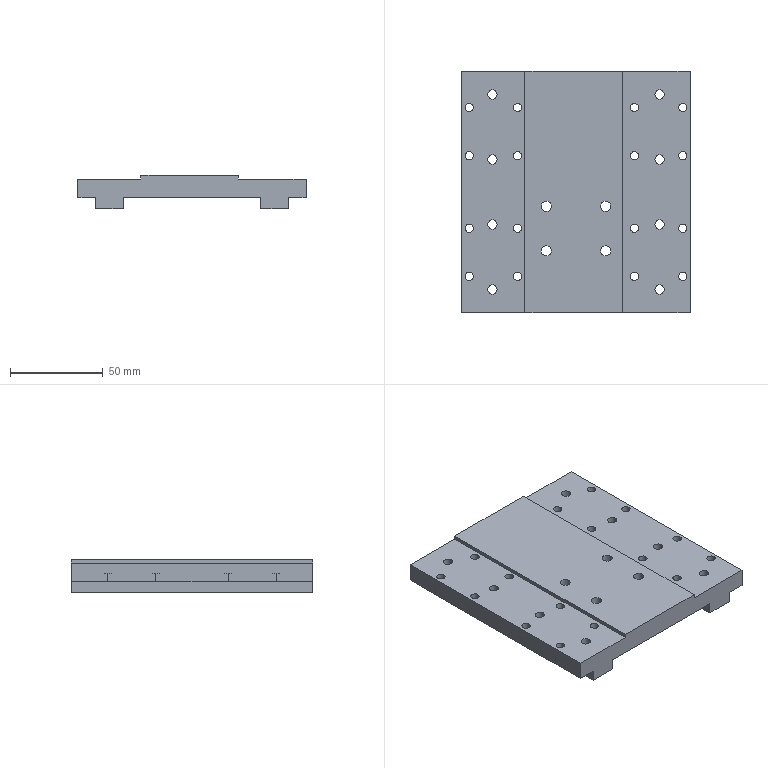NC program | NX | posted with a generic post | part box 123 x 130 x 18 mm
Whole program:
N10 G17 G21 G94 G90
(FLOOR_WALL_1_COPY , TOOL : D10)
N12 T15 M6
N14 G54
N16 G17 G0 G90 X4.33 Y-68. S9500 M3
N18 G43 Z30. H15
N20 Z0.517
N22 G94 G1 Z-0.983 F3000.
N24 X0.866 Y-62.
N26 G3 X0. Y-61.5 R1.
N28 G1 X-65.
N30 Y-57.1
N32 X65.
N34 Y-61.5
N36 X0.
N38 G3 X-0.866 Y-62. R1.
N40 G1 X-4.33 Y-68.
N42 Z0.517
N44 G0 X4.33 Z-0.467
N46 G1 Z-1.967
N48 X0.866 Y-62.
N50 G3 X0. Y-61.5 R1.
N52 G1 X-65.
N54 Y-57.1
N56 X65.
N58 Y-61.5
N60 X0.
N62 G3 X-0.866 Y-62. R1.
N64 G1 X-4.33 Y-68.
N66 Z-0.467
N68 G0 X4.33 Z-1.45
N70 G1 Z-2.95
N72 X0.866 Y-62.
N74 G3 X0. Y-61.5 R1.
N76 G1 X-65.
N78 Y-57.1
N80 X65.
N82 Y-61.5
N84 X0.
N86 G3 X-0.866 Y-62. R1.
N88 G1 X-4.33 Y-68.
N90 Z-1.45
N92 G0 X4.33 Z-2.433
N94 G1 Z-3.933
N96 X0.866 Y-62.
N98 G3 X0. Y-61.5 R1.
N100 G1 X-65.
N102 Y-57.1
N104 X65.
N106 Y-61.5
N108 X0.
N110 G3 X-0.866 Y-62. R1.
N112 G1 X-4.33 Y-68.
N114 Z-2.433
N116 G0 X4.33 Z-3.417
N118 G1 Z-4.917
N120 X0.866 Y-62.
N122 G3 X0. Y-61.5 R1.
N124 G1 X-65.
N126 Y-57.1
N128 X65.
N130 Y-61.5
N132 X0.
N134 G3 X-0.866 Y-62. R1.
N136 G1 X-4.33 Y-68.
N138 Z-3.417
N140 G0 X4.33 Z-4.4
N142 G1 Z-5.9
N144 X0.866 Y-62.
N146 G3 X0. Y-61.5 R1.
N148 G1 X-65.
N150 Y-57.1
N152 X65.
N154 Y-61.5
N156 X0.
N158 G3 X-0.866 Y-62. R1.
N160 G1 X-4.33 Y-68.
N162 Z-4.4
N164 G0 Z30.
N166 X-71.5 Y-4.33
N168 Z0.517
N170 G1 Z-0.983
N172 X-65.5 Y-0.866
N174 G3 X-65. Y0. R1.
N176 G1 Y31.9
N178 X65.
N180 Y-31.9
N182 X-65.
N184 Y0.
N186 X-58.
N188 Y24.9
N190 X58.
N192 Y-24.9
N194 X-58.
N196 Y0.
N198 X-51.
N200 Y17.9
N202 X51.
N204 Y-17.9
N206 X-51.
N208 Y0.
N210 X-44.
N212 Y10.9
N214 X44.
N216 Y-10.9
N218 X-44.
N220 Y0.
N222 X-37.
N224 Y3.9
N226 X37.
N228 Y-3.9
N230 X-37.
N232 Y0.
N234 G3 X-37.5 Y0.866 R1.
N236 G1 Z0.517
N238 G0 X-71.5 Y-4.33 Z-0.467
N240 G1 Z-1.967
N242 X-65.5 Y-0.866
N244 G3 X-65. Y0. R1.
N246 G1 Y31.9
N248 X65.
N250 Y-31.9
N252 X-65.
N254 Y0.
N256 X-58.
N258 Y24.9
N260 X58.
N262 Y-24.9
N264 X-58.
N266 Y0.
N268 X-51.
N270 Y17.9
N272 X51.
N274 Y-17.9
N276 X-51.
N278 Y0.
N280 X-44.
N282 Y10.9
N284 X44.
N286 Y-10.9
N288 X-44.
N290 Y0.
N292 X-37.
N294 Y3.9
N296 X37.
N298 Y-3.9
N300 X-37.
N302 Y0.
N304 G3 X-37.5 Y0.866 R1.
N306 G1 Z-0.467
N308 G0 X-71.5 Y-4.33 Z-1.45
N310 G1 Z-2.95
N312 X-65.5 Y-0.866
N314 G3 X-65. Y0. R1.
N316 G1 Y31.9
N318 X65.
N320 Y-31.9
N322 X-65.
N324 Y0.
N326 X-58.
N328 Y24.9
N330 X58.
N332 Y-24.9
N334 X-58.
N336 Y0.
N338 X-51.
N340 Y17.9
N342 X51.
N344 Y-17.9
N346 X-51.
N348 Y0.
N350 X-44.
N352 Y10.9
N354 X44.
N356 Y-10.9
N358 X-44.
N360 Y0.
N362 X-37.
N364 Y3.9
N366 X37.
N368 Y-3.9
N370 X-37.
N372 Y0.
N374 G3 X-37.5 Y0.866 R1.
N376 G1 Z-1.45
N378 G0 X-71.5 Y-4.33 Z-2.433
N380 G1 Z-3.933
N382 X-65.5 Y-0.866
N384 G3 X-65. Y0. R1.
N386 G1 Y31.9
N388 X65.
N390 Y-31.9
N392 X-65.
N394 Y0.
N396 X-58.
N398 Y24.9
N400 X58.
N402 Y-24.9
N404 X-58.
N406 Y0.
N408 X-51.
N410 Y17.9
N412 X51.
N414 Y-17.9
N416 X-51.
N418 Y0.
N420 X-44.
N422 Y10.9
N424 X44.
N426 Y-10.9
N428 X-44.
N430 Y0.
N432 X-37.
N434 Y3.9
N436 X37.
N438 Y-3.9
N440 X-37.
N442 Y0.
N444 G3 X-37.5 Y0.866 R1.
N446 G1 Z-2.433
N448 G0 X-71.5 Y-4.33 Z-3.417
N450 G1 Z-4.917
N452 X-65.5 Y-0.866
N454 G3 X-65. Y0. R1.
N456 G1 Y31.9
N458 X65.
N460 Y-31.9
N462 X-65.
N464 Y0.
N466 X-58.
N468 Y24.9
N470 X58.
N472 Y-24.9
N474 X-58.
N476 Y0.
N478 X-51.
N480 Y17.9
N482 X51.
N484 Y-17.9
N486 X-51.
N488 Y0.
N490 X-44.
N492 Y10.9
N494 X44.
N496 Y-10.9
N498 X-44.
N500 Y0.
N502 X-37.
N504 Y3.9
N506 X37.
N508 Y-3.9
N510 X-37.
N512 Y0.
N514 G3 X-37.5 Y0.866 R1.
N516 G1 Z-3.417
N518 G0 X-71.5 Y-4.33 Z-4.4
N520 G1 Z-5.9
N522 X-65.5 Y-0.866
N524 G3 X-65. Y0. R1.
N526 G1 Y31.9
N528 X65.
N530 Y-31.9
N532 X-65.
N534 Y0.
N536 X-58.
N538 Y24.9
N540 X58.
N542 Y-24.9
N544 X-58.
N546 Y0.
N548 X-51.
N550 Y17.9
N552 X51.
N554 Y-17.9
N556 X-51.
N558 Y0.
N560 X-44.
N562 Y10.9
N564 X44.
N566 Y-10.9
N568 X-44.
N570 Y0.
N572 X-37.
N574 Y3.9
N576 X37.
N578 Y-3.9
N580 X-37.
N582 Y0.
N584 G3 X-37.5 Y0.866 R1.
N586 G1 Z-4.4
N588 G0 Z30.
N590 X-4.33 Y68.
N592 Z0.517
N594 G1 Z-0.983
N596 X-0.866 Y62.
N598 G3 X0. Y61.5 R1.
N600 G1 X65.
N602 Y57.1
N604 X-65.
N606 Y61.5
N608 X0.
N610 G3 X0.866 Y62. R1.
N612 G1 X4.33 Y68.
N614 Z0.517
N616 G0 X-4.33 Z-0.467
N618 G1 Z-1.967
N620 X-0.866 Y62.
N622 G3 X0. Y61.5 R1.
N624 G1 X65.
N626 Y57.1
N628 X-65.
N630 Y61.5
N632 X0.
N634 G3 X0.866 Y62. R1.
N636 G1 X4.33 Y68.
N638 Z-0.467
N640 G0 X-4.33 Z-1.45
N642 G1 Z-2.95
N644 X-0.866 Y62.
N646 G3 X0. Y61.5 R1.
N648 G1 X65.
N650 Y57.1
N652 X-65.
N654 Y61.5
N656 X0.
N658 G3 X0.866 Y62. R1.
N660 G1 X4.33 Y68.
N662 Z-1.45
N664 G0 X-4.33 Z-2.433
N666 G1 Z-3.933
N668 X-0.866 Y62.
N670 G3 X0. Y61.5 R1.
N672 G1 X65.
N674 Y57.1
N676 X-65.
N678 Y61.5
N680 X0.
N682 G3 X0.866 Y62. R1.
N684 G1 X4.33 Y68.
N686 Z-2.433
N688 G0 X-4.33 Z-3.417
N690 G1 Z-4.917
N692 X-0.866 Y62.
N694 G3 X0. Y61.5 R1.
N696 G1 X65.
N698 Y57.1
N700 X-65.
N702 Y61.5
N704 X0.
N706 G3 X0.866 Y62. R1.
N708 G1 X4.33 Y68.
N710 Z-3.417
N712 G0 X-4.33 Z-4.4
N714 G1 Z-5.9
N716 X-0.866 Y62.
N718 G3 X0. Y61.5 R1.
N720 G1 X65.
N722 Y57.1
N724 X-65.
N726 Y61.5
N728 X0.
N730 G3 X0.866 Y62. R1.
N732 G1 X4.33 Y68.
N734 Z-4.4
N736 G0 Z30.
N738 M5
(FLOOR_WALL_COPY_COPY , TOOL : D10JING)
N740 T14 M6
N742 G54
N744 G17 G0 G90 X-71.5 Y63.097 S9500 M3
N746 G43 Z30. H14
N748 Z-4.5
N750 G94 G1 Z-6. F1500.
N752 X-70.866 Y61.999
N754 G3 X-70. Y61.499 R1.
N756 G1 X70.
N758 Y57.5
N760 X-70.
N762 G2 X-70.866 Y58. R1.
N764 G1 X-71.5 Y59.098
N766 Z-4.5
N768 G0 Y58.598
N770 G1 Z-6.
N772 X-70.866 Y57.5
N774 G3 X-70. Y57. R1.
N776 G1 X70.
N778 G3 X70.866 Y57.5 R1.
N780 G1 X71.5 Y58.598
N782 Z-4.5
N784 G0 Z30.
N786 X-71.5 Y30.999
N788 Z-4.5
N790 G1 Z-6.
N792 X-69.134
N794 G3 X-70. Y31.499 R1.
N796 G1 X70.
N798 Y26.653
N800 X-70.
N802 Y21.807
N804 X70.
N806 Y16.961
N808 X-70.
N810 Y12.115
N812 X70.
N814 Y7.269
N816 X-70.
N818 Y2.423
N820 X70.
N822 Y-2.424
N824 X-70.
N826 Y-7.27
N828 X70.
N830 Y-12.116
N832 X-70.
N834 Y-16.962
N836 X70.
N838 Y-21.808
N840 X-70.
N842 Y-26.654
N844 X70.
N846 Y-31.5
N848 X-70.
N850 G2 X-70.866 Y-31. R1.
N852 G1 X-71.5 Y-29.902
N854 Z-4.5
N856 G0 Y-30.402
N858 G1 Z-6.
N860 X-70.866 Y-31.5
N862 G3 X-70. Y-32. R1.
N864 G1 X70.
N866 G3 X70.866 Y-31.5 R1.
N868 G1 X71.5 Y-30.402
N870 Z-4.5
N872 G0 Y30.402
N874 G1 Z-6.
N876 X70.866 Y31.5
N878 G3 X70. Y32. R1.
N880 G1 X-70.
N882 G3 X-70.866 Y31.5 R1.
N884 G1 X-71.5 Y30.402
N886 Z-4.5
N888 G0 Z30.
N890 X71.5 Y-63.097
N892 Z-4.5
N894 G1 Z-6.
N896 X70.866 Y-61.999
N898 G3 X70. Y-61.499 R1.
N900 G1 X-70.
N902 Y-57.5
N904 X70.
N906 G2 X70.866 Y-58. R1.
N908 G1 X71.5 Y-59.098
N910 Z-4.5
N912 G0 Y-58.598
N914 G1 Z-6.
N916 X70.866 Y-57.5
N918 G3 X70. Y-57. R1.
N920 G1 X-70.
N922 G3 X-70.866 Y-57.5 R1.
N924 G1 X-71.5 Y-58.598
N926 Z-4.5
N928 G0 Z30.
N930 M5
(HOLE_MILLING , TOOL : D6)
N932 T12 M6
N934 G54
N936 G17 G0 G90 X-45.5 Y31.5 S9500 M3
N938 G43 Z30. H12
N940 Z-5.5
N942 G94 G3 X-45. Y32. R0.5 F1600.
N944 X-45.5 Y32.5 R0.5
N946 X-45.5 Y32.5 Z-6. I0. J-1.
N948 X-45.5 Y32.5 Z-6.5 I0. J-1.
N950 X-45.5 Y32.5 Z-7. I0. J-1.
N952 X-45.5 Y32.5 Z-7.5 I0. J-1.
N954 X-45.5 Y32.5 Z-8. I0. J-1.
N956 X-45.5 Y32.5 Z-8.5 I0. J-1.
N958 X-45.5 Y32.5 Z-9. I0. J-1.
N960 X-45.5 Y32.5 Z-9.5 I0. J-1.
N962 X-45.5 Y32.5 Z-10. I0. J-1.
N964 X-45.5 Y32.5 Z-10.5 I0. J-1.
N966 X-46.5 Y31.5 R1.
N968 X-45.5 Y32.5 R-1.
N970 X-46. Y32. R0.5
N972 X-45.5 Y31.5 R0.5
N974 G0 Z30.
N976 Y57.5
N978 Z-5.5
N980 G3 X-45. Y58. R0.5
N982 X-45.5 Y58.5 R0.5
N984 X-45.5 Y58.5 Z-6. I0. J-1.
N986 X-45.5 Y58.5 Z-6.5 I0. J-1.
N988 X-45.5 Y58.5 Z-7. I0. J-1.
N990 X-45.5 Y58.5 Z-7.5 I0. J-1.
N992 X-45.5 Y58.5 Z-8. I0. J-1.
N994 X-45.5 Y58.5 Z-8.5 I0. J-1.
N996 X-45.5 Y58.5 Z-9. I0. J-1.
N998 X-45.5 Y58.5 Z-9.5 I0. J-1.
N1000 X-45.5 Y58.5 Z-10. I0. J-1.
N1002 X-45.5 Y58.5 Z-10.5 I0. J-1.
N1004 X-46.5 Y57.5 R1.
N1006 X-45.5 Y58.5 R-1.
N1008 X-46. Y58. R0.5
N1010 X-45.5 Y57.5 R0.5
N1012 G0 Z30.
N1014 X-19.5
N1016 Z-5.5
N1018 G3 X-19. Y58. R0.5
N1020 X-19.5 Y58.5 R0.5
N1022 X-19.5 Y58.5 Z-6. I0. J-1.
N1024 X-19.5 Y58.5 Z-6.5 I0. J-1.
N1026 X-19.5 Y58.5 Z-7. I0. J-1.
N1028 X-19.5 Y58.5 Z-7.5 I0. J-1.
N1030 X-19.5 Y58.5 Z-8. I0. J-1.
N1032 X-19.5 Y58.5 Z-8.5 I0. J-1.
N1034 X-19.5 Y58.5 Z-9. I0. J-1.
N1036 X-19.5 Y58.5 Z-9.5 I0. J-1.
N1038 X-19.5 Y58.5 Z-10. I0. J-1.
N1040 X-19.5 Y58.5 Z-10.5 I0. J-1.
N1042 X-20.5 Y57.5 R1.
N1044 X-19.5 Y58.5 R-1.
N1046 X-20. Y58. R0.5
N1048 X-19.5 Y57.5 R0.5
N1050 G0 Z30.
N1052 X19.5
N1054 Z-5.5
N1056 G3 X20. Y58. R0.5
N1058 X19.5 Y58.5 R0.5
N1060 X19.5 Y58.5 Z-6. I0. J-1.
N1062 X19.5 Y58.5 Z-6.5 I0. J-1.
N1064 X19.5 Y58.5 Z-7. I0. J-1.
N1066 X19.5 Y58.5 Z-7.5 I0. J-1.
N1068 X19.5 Y58.5 Z-8. I0. J-1.
N1070 X19.5 Y58.5 Z-8.5 I0. J-1.
N1072 X19.5 Y58.5 Z-9. I0. J-1.
N1074 X19.5 Y58.5 Z-9.5 I0. J-1.
N1076 X19.5 Y58.5 Z-10. I0. J-1.
N1078 X19.5 Y58.5 Z-10.5 I0. J-1.
N1080 X18.5 Y57.5 R1.
N1082 X19.5 Y58.5 R-1.
N1084 X19. Y58. R0.5
N1086 X19.5 Y57.5 R0.5
N1088 G0 Z30.
N1090 X45.5
N1092 Z-5.5
N1094 G3 X46. Y58. R0.5
N1096 X45.5 Y58.5 R0.5
N1098 X45.5 Y58.5 Z-6. I0. J-1.
N1100 X45.5 Y58.5 Z-6.5 I0. J-1.
N1102 X45.5 Y58.5 Z-7. I0. J-1.
N1104 X45.5 Y58.5 Z-7.5 I0. J-1.
N1106 X45.5 Y58.5 Z-8. I0. J-1.
N1108 X45.5 Y58.5 Z-8.5 I0. J-1.
N1110 X45.5 Y58.5 Z-9. I0. J-1.
N1112 X45.5 Y58.5 Z-9.5 I0. J-1.
N1114 X45.5 Y58.5 Z-10. I0. J-1.
N1116 X45.5 Y58.5 Z-10.5 I0. J-1.
N1118 X44.5 Y57.5 R1.
N1120 X45.5 Y58.5 R-1.
N1122 X45. Y58. R0.5
N1124 X45.5 Y57.5 R0.5
N1126 G0 Z30.
N1128 Y31.5
N1130 Z-5.5
N1132 G3 X46. Y32. R0.5
N1134 X45.5 Y32.5 R0.5
N1136 X45.5 Y32.5 Z-6. I0. J-1.
N1138 X45.5 Y32.5 Z-6.5 I0. J-1.
N1140 X45.5 Y32.5 Z-7. I0. J-1.
N1142 X45.5 Y32.5 Z-7.5 I0. J-1.
N1144 X45.5 Y32.5 Z-8. I0. J-1.
N1146 X45.5 Y32.5 Z-8.5 I0. J-1.
N1148 X45.5 Y32.5 Z-9. I0. J-1.
N1150 X45.5 Y32.5 Z-9.5 I0. J-1.
N1152 X45.5 Y32.5 Z-10. I0. J-1.
N1154 X45.5 Y32.5 Z-10.5 I0. J-1.
N1156 X44.5 Y31.5 R1.
N1158 X45.5 Y32.5 R-1.
N1160 X45. Y32. R0.5
N1162 X45.5 Y31.5 R0.5
N1164 G0 Z30.
N1166 X19.5
N1168 Z-5.5
N1170 G3 X20. Y32. R0.5
N1172 X19.5 Y32.5 R0.5
N1174 X19.5 Y32.5 Z-6. I0. J-1.
N1176 X19.5 Y32.5 Z-6.5 I0. J-1.
N1178 X19.5 Y32.5 Z-7. I0. J-1.
N1180 X19.5 Y32.5 Z-7.5 I0. J-1.
N1182 X19.5 Y32.5 Z-8. I0. J-1.
N1184 X19.5 Y32.5 Z-8.5 I0. J-1.
N1186 X19.5 Y32.5 Z-9. I0. J-1.
N1188 X19.5 Y32.5 Z-9.5 I0. J-1.
N1190 X19.5 Y32.5 Z-10. I0. J-1.
N1192 X19.5 Y32.5 Z-10.5 I0. J-1.
N1194 X18.5 Y31.5 R1.
N1196 X19.5 Y32.5 R-1.
N1198 X19. Y32. R0.5
N1200 X19.5 Y31.5 R0.5
N1202 G0 Z30.
N1204 X-7.7 Y16.
N1206 Z-5.5
N1208 G3 X-6.7 Y17. R1.
N1210 X-7.7 Y18. R1.
N1212 X-7.7 Y18. Z-6. I0. J-2.
N1214 X-7.7 Y18. Z-6.5 I0. J-2.
N1216 X-7.7 Y18. Z-7. I0. J-2.
N1218 X-7.7 Y18. Z-7.5 I0. J-2.
N1220 X-7.7 Y18. Z-8. I0. J-2.
N1222 X-7.7 Y18. Z-8.5 I0. J-2.
N1224 X-7.7 Y18. Z-9. I0. J-2.
N1226 X-7.7 Y18. Z-9.5 I0. J-2.
N1228 X-7.7 Y18. Z-10. I0. J-2.
N1230 X-7.7 Y18. Z-10.5 I0. J-2.
N1232 X-7.7 Y18. Z-11. I0. J-2.
N1234 X-7.7 Y18. Z-11.5 I0. J-2.
N1236 X-9.7 Y16. R2.
N1238 X-7.7 Y18. R-2.
N1240 X-8.7 Y17. R1.
N1242 X-7.7 Y16. R1.
N1244 G0 Z30.
N1246 X-19.5 Y31.5
N1248 Z-5.5
N1250 G3 X-19. Y32. R0.5
N1252 X-19.5 Y32.5 R0.5
N1254 X-19.5 Y32.5 Z-6. I0. J-1.
N1256 X-19.5 Y32.5 Z-6.5 I0. J-1.
N1258 X-19.5 Y32.5 Z-7. I0. J-1.
N1260 X-19.5 Y32.5 Z-7.5 I0. J-1.
N1262 X-19.5 Y32.5 Z-8. I0. J-1.
N1264 X-19.5 Y32.5 Z-8.5 I0. J-1.
N1266 X-19.5 Y32.5 Z-9. I0. J-1.
N1268 X-19.5 Y32.5 Z-9.5 I0. J-1.
N1270 X-19.5 Y32.5 Z-10. I0. J-1.
N1272 X-19.5 Y32.5 Z-10.5 I0. J-1.
N1274 X-20.5 Y31.5 R1.
N1276 X-19.5 Y32.5 R-1.
N1278 X-20. Y32. R0.5
N1280 X-19.5 Y31.5 R0.5
N1282 G0 Z30.
N1284 X-31.7 Y16.
N1286 Z-5.5
N1288 G3 X-30.7 Y17. R1.
N1290 X-31.7 Y18. R1.
N1292 X-31.7 Y18. Z-6. I0. J-2.
N1294 X-31.7 Y18. Z-6.5 I0. J-2.
N1296 X-31.7 Y18. Z-7. I0. J-2.
N1298 X-31.7 Y18. Z-7.5 I0. J-2.
N1300 X-31.7 Y18. Z-8. I0. J-2.
N1302 X-31.7 Y18. Z-8.5 I0. J-2.
N1304 X-31.7 Y18. Z-9. I0. J-2.
N1306 X-31.7 Y18. Z-9.5 I0. J-2.
N1308 X-31.7 Y18. Z-10. I0. J-2.
N1310 X-31.7 Y18. Z-10.5 I0. J-2.
N1312 X-31.7 Y18. Z-11. I0. J-2.
N1314 X-31.7 Y18. Z-11.5 I0. J-2.
N1316 X-33.7 Y16. R2.
N1318 X-31.7 Y18. R-2.
N1320 X-32.7 Y17. R1.
N1322 X-31.7 Y16. R1.
N1324 G0 Z30.
N1326 Y-16.
N1328 Z-5.5
N1330 G3 X-30.7 Y-15. R1.
N1332 X-31.7 Y-14. R1.
N1334 X-31.7 Y-14. Z-6. I0. J-2.
N1336 X-31.7 Y-14. Z-6.5 I0. J-2.
N1338 X-31.7 Y-14. Z-7. I0. J-2.
N1340 X-31.7 Y-14. Z-7.5 I0. J-2.
N1342 X-31.7 Y-14. Z-8. I0. J-2.
N1344 X-31.7 Y-14. Z-8.5 I0. J-2.
N1346 X-31.7 Y-14. Z-9. I0. J-2.
N1348 X-31.7 Y-14. Z-9.5 I0. J-2.
N1350 X-31.7 Y-14. Z-10. I0. J-2.
N1352 X-31.7 Y-14. Z-10.5 I0. J-2.
N1354 X-31.7 Y-14. Z-11. I0. J-2.
N1356 X-31.7 Y-14. Z-11.5 I0. J-2.
N1358 X-33.7 Y-16. R2.
N1360 X-31.7 Y-14. R-2.
N1362 X-32.7 Y-15. R1.
N1364 X-31.7 Y-16. R1.
N1366 G0 Z30.
N1368 X-45.5 Y-31.5
N1370 Z-5.5
N1372 G3 X-45. Y-31. R0.5
N1374 X-45.5 Y-30.5 R0.5
N1376 X-45.5 Y-30.5 Z-6. I0. J-1.
N1378 X-45.5 Y-30.5 Z-6.5 I0. J-1.
N1380 X-45.5 Y-30.5 Z-7. I0. J-1.
N1382 X-45.5 Y-30.5 Z-7.5 I0. J-1.
N1384 X-45.5 Y-30.5 Z-8. I0. J-1.
N1386 X-45.5 Y-30.5 Z-8.5 I0. J-1.
N1388 X-45.5 Y-30.5 Z-9. I0. J-1.
N1390 X-45.5 Y-30.5 Z-9.5 I0. J-1.
N1392 X-45.5 Y-30.5 Z-10. I0. J-1.
N1394 X-45.5 Y-30.5 Z-10.5 I0. J-1.
N1396 X-46.5 Y-31.5 R1.
N1398 X-45.5 Y-30.5 R-1.
N1400 X-46. Y-31. R0.5
N1402 X-45.5 Y-31.5 R0.5
N1404 G0 Z30.
N1406 Y-57.5
N1408 Z-5.5
N1410 G3 X-45. Y-57. R0.5
N1412 X-45.5 Y-56.5 R0.5
N1414 X-45.5 Y-56.5 Z-6. I0. J-1.
N1416 X-45.5 Y-56.5 Z-6.5 I0. J-1.
N1418 X-45.5 Y-56.5 Z-7. I0. J-1.
N1420 X-45.5 Y-56.5 Z-7.5 I0. J-1.
N1422 X-45.5 Y-56.5 Z-8. I0. J-1.
N1424 X-45.5 Y-56.5 Z-8.5 I0. J-1.
N1426 X-45.5 Y-56.5 Z-9. I0. J-1.
N1428 X-45.5 Y-56.5 Z-9.5 I0. J-1.
N1430 X-45.5 Y-56.5 Z-10. I0. J-1.
N1432 X-45.5 Y-56.5 Z-10.5 I0. J-1.
N1434 X-46.5 Y-57.5 R1.
N1436 X-45.5 Y-56.5 R-1.
N1438 X-46. Y-57. R0.5
N1440 X-45.5 Y-57.5 R0.5
N1442 G0 Z30.
N1444 X-19.5
N1446 Z-5.5
N1448 G3 X-19. Y-57. R0.5
N1450 X-19.5 Y-56.5 R0.5
N1452 X-19.5 Y-56.5 Z-6. I0. J-1.
N1454 X-19.5 Y-56.5 Z-6.5 I0. J-1.
N1456 X-19.5 Y-56.5 Z-7. I0. J-1.
N1458 X-19.5 Y-56.5 Z-7.5 I0. J-1.
N1460 X-19.5 Y-56.5 Z-8. I0. J-1.
N1462 X-19.5 Y-56.5 Z-8.5 I0. J-1.
N1464 X-19.5 Y-56.5 Z-9. I0. J-1.
N1466 X-19.5 Y-56.5 Z-9.5 I0. J-1.
N1468 X-19.5 Y-56.5 Z-10. I0. J-1.
N1470 X-19.5 Y-56.5 Z-10.5 I0. J-1.
N1472 X-20.5 Y-57.5 R1.
N1474 X-19.5 Y-56.5 R-1.
N1476 X-20. Y-57. R0.5
N1478 X-19.5 Y-57.5 R0.5
N1480 G0 Z30.
N1482 Y-31.5
N1484 Z-5.5
N1486 G3 X-19. Y-31. R0.5
N1488 X-19.5 Y-30.5 R0.5
N1490 X-19.5 Y-30.5 Z-6. I0. J-1.
N1492 X-19.5 Y-30.5 Z-6.5 I0. J-1.
N1494 X-19.5 Y-30.5 Z-7. I0. J-1.
N1496 X-19.5 Y-30.5 Z-7.5 I0. J-1.
N1498 X-19.5 Y-30.5 Z-8. I0. J-1.
N1500 X-19.5 Y-30.5 Z-8.5 I0. J-1.
N1502 X-19.5 Y-30.5 Z-9. I0. J-1.
N1504 X-19.5 Y-30.5 Z-9.5 I0. J-1.
N1506 X-19.5 Y-30.5 Z-10. I0. J-1.
N1508 X-19.5 Y-30.5 Z-10.5 I0. J-1.
N1510 X-20.5 Y-31.5 R1.
N1512 X-19.5 Y-30.5 R-1.
N1514 X-20. Y-31. R0.5
N1516 X-19.5 Y-31.5 R0.5
N1518 G0 Z30.
N1520 X-7.7 Y-16.
N1522 Z-5.5
N1524 G3 X-6.7 Y-15. R1.
N1526 X-7.7 Y-14. R1.
N1528 X-7.7 Y-14. Z-6. I0. J-2.
N1530 X-7.7 Y-14. Z-6.5 I0. J-2.
N1532 X-7.7 Y-14. Z-7. I0. J-2.
N1534 X-7.7 Y-14. Z-7.5 I0. J-2.
N1536 X-7.7 Y-14. Z-8. I0. J-2.
N1538 X-7.7 Y-14. Z-8.5 I0. J-2.
N1540 X-7.7 Y-14. Z-9. I0. J-2.
N1542 X-7.7 Y-14. Z-9.5 I0. J-2.
N1544 X-7.7 Y-14. Z-10. I0. J-2.
N1546 X-7.7 Y-14. Z-10.5 I0. J-2.
N1548 X-7.7 Y-14. Z-11. I0. J-2.
N1550 X-7.7 Y-14. Z-11.5 I0. J-2.
N1552 X-9.7 Y-16. R2.
N1554 X-7.7 Y-14. R-2.
N1556 X-8.7 Y-15. R1.
N1558 X-7.7 Y-16. R1.
N1560 G0 Z30.
N1562 X19.5 Y-31.5
N1564 Z-5.5
N1566 G3 X20. Y-31. R0.5
N1568 X19.5 Y-30.5 R0.5
N1570 X19.5 Y-30.5 Z-6. I0. J-1.
N1572 X19.5 Y-30.5 Z-6.5 I0. J-1.
N1574 X19.5 Y-30.5 Z-7. I0. J-1.
N1576 X19.5 Y-30.5 Z-7.5 I0. J-1.
N1578 X19.5 Y-30.5 Z-8. I0. J-1.
N1580 X19.5 Y-30.5 Z-8.5 I0. J-1.
N1582 X19.5 Y-30.5 Z-9. I0. J-1.
N1584 X19.5 Y-30.5 Z-9.5 I0. J-1.
N1586 X19.5 Y-30.5 Z-10. I0. J-1.
N1588 X19.5 Y-30.5 Z-10.5 I0. J-1.
N1590 X18.5 Y-31.5 R1.
N1592 X19.5 Y-30.5 R-1.
N1594 X19. Y-31. R0.5
N1596 X19.5 Y-31.5 R0.5
N1598 G0 Z30.
N1600 Y-57.5
N1602 Z-5.5
N1604 G3 X20. Y-57. R0.5
N1606 X19.5 Y-56.5 R0.5
N1608 X19.5 Y-56.5 Z-6. I0. J-1.
N1610 X19.5 Y-56.5 Z-6.5 I0. J-1.
N1612 X19.5 Y-56.5 Z-7. I0. J-1.
N1614 X19.5 Y-56.5 Z-7.5 I0. J-1.
N1616 X19.5 Y-56.5 Z-8. I0. J-1.
N1618 X19.5 Y-56.5 Z-8.5 I0. J-1.
N1620 X19.5 Y-56.5 Z-9. I0. J-1.
N1622 X19.5 Y-56.5 Z-9.5 I0. J-1.
N1624 X19.5 Y-56.5 Z-10. I0. J-1.
N1626 X19.5 Y-56.5 Z-10.5 I0. J-1.
N1628 X18.5 Y-57.5 R1.
N1630 X19.5 Y-56.5 R-1.
N1632 X19. Y-57. R0.5
N1634 X19.5 Y-57.5 R0.5
N1636 G0 Z30.
N1638 X45.5
N1640 Z-5.5
N1642 G3 X46. Y-57. R0.5
N1644 X45.5 Y-56.5 R0.5
N1646 X45.5 Y-56.5 Z-6. I0. J-1.
N1648 X45.5 Y-56.5 Z-6.5 I0. J-1.
N1650 X45.5 Y-56.5 Z-7. I0. J-1.
N1652 X45.5 Y-56.5 Z-7.5 I0. J-1.
N1654 X45.5 Y-56.5 Z-8. I0. J-1.
N1656 X45.5 Y-56.5 Z-8.5 I0. J-1.
N1658 X45.5 Y-56.5 Z-9. I0. J-1.
N1660 X45.5 Y-56.5 Z-9.5 I0. J-1.
N1662 X45.5 Y-56.5 Z-10. I0. J-1.
N1664 X45.5 Y-56.5 Z-10.5 I0. J-1.
N1666 X44.5 Y-57.5 R1.
N1668 X45.5 Y-56.5 R-1.
N1670 X45. Y-57. R0.5
N1672 X45.5 Y-57.5 R0.5
N1674 G0 Z30.
N1676 Y-31.5
N1678 Z-5.5
N1680 G3 X46. Y-31. R0.5
N1682 X45.5 Y-30.5 R0.5
N1684 X45.5 Y-30.5 Z-6. I0. J-1.
N1686 X45.5 Y-30.5 Z-6.5 I0. J-1.
N1688 X45.5 Y-30.5 Z-7. I0. J-1.
N1690 X45.5 Y-30.5 Z-7.5 I0. J-1.
N1692 X45.5 Y-30.5 Z-8. I0. J-1.
N1694 X45.5 Y-30.5 Z-8.5 I0. J-1.
N1696 X45.5 Y-30.5 Z-9. I0. J-1.
N1698 X45.5 Y-30.5 Z-9.5 I0. J-1.
N1700 X45.5 Y-30.5 Z-10. I0. J-1.
N1702 X45.5 Y-30.5 Z-10.5 I0. J-1.
N1704 X44.5 Y-31.5 R1.
N1706 X45.5 Y-30.5 R-1.
N1708 X45. Y-31. R0.5
N1710 X45.5 Y-31.5 R0.5
N1712 G0 Z30.
N1714 M5
(HOLE_MILLING_COPY , TOOL : D4)
N1716 T11 M6
N1718 G54
N1720 G17 G0 G90 X0. Y45. S9500 M3
N1722 G43 Z30. H11
N1724 Z0.5
N1726 G94 G3 X0.45 Y45.45 R0.45 F1600.
N1728 X0. Y45.9 R0.45
N1730 X0. Y45.9 Z0.2 I0. J-0.9
N1732 X0. Y45.9 Z-0.1 I0. J-0.9
N1734 X0. Y45.9 Z-0.4 I0. J-0.9
N1736 X0. Y45.9 Z-0.7 I0. J-0.9
N1738 X0. Y45.9 Z-1. I0. J-0.9
N1740 X0. Y45.9 Z-1.3 I0. J-0.9
N1742 X0. Y45.9 Z-1.6 I0. J-0.9
N1744 X0. Y45.9 Z-1.9 I0. J-0.9
N1746 X0. Y45.9 Z-2.2 I0. J-0.9
N1748 X0. Y45.9 Z-2.5 I0. J-0.9
N1750 X0. Y45.9 Z-2.8 I0. J-0.9
N1752 X0. Y45.9 Z-3.1 I0. J-0.9
N1754 X0. Y45.9 Z-3.4 I0. J-0.9
N1756 X0. Y45.9 Z-3.7 I0. J-0.9
N1758 X0. Y45.9 Z-4. I0. J-0.9
N1760 X0. Y45.9 Z-4.3 I0. J-0.9
N1762 X0. Y45.9 Z-4.6 I0. J-0.9
N1764 X0. Y45.9 Z-4.9 I0. J-0.9
N1766 X0. Y45.9 Z-5.2 I0. J-0.9
N1768 X0. Y45.9 Z-5.5 I0. J-0.9
N1770 X0. Y45.9 Z-5.8 I0. J-0.9
N1772 X0. Y45.9 Z-6.1 I0. J-0.9
N1774 X0. Y45.9 Z-6.4 I0. J-0.9
N1776 X0. Y45.9 Z-6.7 I0. J-0.9
N1778 X0. Y45.9 Z-7. I0. J-0.9
N1780 X0. Y45.9 Z-7.3 I0. J-0.9
N1782 X0. Y45.9 Z-7.6 I0. J-0.9
N1784 X0. Y45.9 Z-7.9 I0. J-0.9
N1786 X0. Y45.9 Z-8.2 I0. J-0.9
N1788 X0. Y45.9 Z-8.5 I0. J-0.9
N1790 X0. Y45.9 Z-8.8 I0. J-0.9
N1792 X0. Y45.9 Z-9.1 I0. J-0.9
N1794 X0. Y45.9 Z-9.4 I0. J-0.9
N1796 X0. Y45.9 Z-9.7 I0. J-0.9
N1798 X0. Y45.9 Z-10. I0. J-0.9
N1800 X-0.9 Y45. R0.9
N1802 X0. Y45.9 R-0.9
N1804 X-0.45 Y45.45 R0.45
N1806 X0. Y45. R0.45
N1808 G0 Z30.
N1810 Y-45.
N1812 Z0.5
N1814 G3 X0.45 Y-44.55 R0.45
N1816 X0. Y-44.1 R0.45
N1818 X0. Y-44.1 Z0.2 I0. J-0.9
N1820 X0. Y-44.1 Z-0.1 I0. J-0.9
N1822 X0. Y-44.1 Z-0.4 I0. J-0.9
N1824 X0. Y-44.1 Z-0.7 I0. J-0.9
N1826 X0. Y-44.1 Z-1. I0. J-0.9
N1828 X0. Y-44.1 Z-1.3 I0. J-0.9
N1830 X0. Y-44.1 Z-1.6 I0. J-0.9
N1832 X0. Y-44.1 Z-1.9 I0. J-0.9
N1834 X0. Y-44.1 Z-2.2 I0. J-0.9
N1836 X0. Y-44.1 Z-2.5 I0. J-0.9
N1838 X0. Y-44.1 Z-2.8 I0. J-0.9
N1840 X0. Y-44.1 Z-3.1 I0. J-0.9
N1842 X0. Y-44.1 Z-3.4 I0. J-0.9
N1844 X0. Y-44.1 Z-3.7 I0. J-0.9
N1846 X0. Y-44.1 Z-4. I0. J-0.9
N1848 X0. Y-44.1 Z-4.3 I0. J-0.9
N1850 X0. Y-44.1 Z-4.6 I0. J-0.9
N1852 X0. Y-44.1 Z-4.9 I0. J-0.9
N1854 X0. Y-44.1 Z-5.2 I0. J-0.9
N1856 X0. Y-44.1 Z-5.5 I0. J-0.9
N1858 X0. Y-44.1 Z-5.8 I0. J-0.9
N1860 X0. Y-44.1 Z-6.1 I0. J-0.9
N1862 X0. Y-44.1 Z-6.4 I0. J-0.9
N1864 X0. Y-44.1 Z-6.7 I0. J-0.9
N1866 X0. Y-44.1 Z-7. I0. J-0.9
N1868 X0. Y-44.1 Z-7.3 I0. J-0.9
N1870 X0. Y-44.1 Z-7.6 I0. J-0.9
N1872 X0. Y-44.1 Z-7.9 I0. J-0.9
N1874 X0. Y-44.1 Z-8.2 I0. J-0.9
N1876 X0. Y-44.1 Z-8.5 I0. J-0.9
N1878 X0. Y-44.1 Z-8.8 I0. J-0.9
N1880 X0. Y-44.1 Z-9.1 I0. J-0.9
N1882 X0. Y-44.1 Z-9.4 I0. J-0.9
N1884 X0. Y-44.1 Z-9.7 I0. J-0.9
N1886 X0. Y-44.1 Z-10. I0. J-0.9
N1888 X-0.9 Y-45. R0.9
N1890 X0. Y-44.1 R-0.9
N1892 X-0.45 Y-44.55 R0.45
N1894 X0. Y-45. R0.45
N1896 G0 Z30.
N1898 M5
(PLANAR_MILL_COPY_COPY_COPY_COPY_1 , TOOL : D6A45)
N1900 T01 M6
N1902 G54
N1904 G17 G0 G90 X53.366 Y46.1 S9500 M3
N1906 G43 Z30. H1
N1908 Z0.5
N1910 G94 G1 Z-1. F1250.
N1912 G3 X52.5 Y46.6 R1.
N1914 X50.9 Y45. R1.6
N1916 X52.5 Y46.6 R-1.6
N1918 X51.634 Y46.1 R1.
N1920 G1 Z0.5
N1922 G0 Z30.
N1924 X18.366
N1926 Z0.5
N1928 G1 Z-1.
N1930 G3 X17.5 Y46.6 R1.
N1932 X15.9 Y45. R1.6
N1934 X17.5 Y46.6 R-1.6
N1936 X16.634 Y46.1 R1.
N1938 G1 Z0.5
N1940 G0 Z30.
N1942 X0.866 Y46.6
N1944 Z0.5
N1946 G1 Z-1.
N1948 G3 X0. Y47.1 R1.
N1950 X-2.1 Y45. R2.1
N1952 X0. Y47.1 R-2.1
N1954 X-0.866 Y46.6 R1.
N1956 G1 Z0.5
N1958 G0 Z30.
N1960 Y53.4
N1962 Z0.5
N1964 G1 Z-1.
N1966 G3 X0. Y52.9 R1.
N1968 G1 X65.
N1970 G2 X65.9 Y52. R0.9
N1972 G1 Y37.
N1974 G2 X65. Y36.1 R0.9
N1976 G1 X-65.
N1978 G2 X-65.9 Y37. R0.9
N1980 G1 Y52.
N1982 G2 X-65. Y52.9 R0.9
N1984 G1 X0.
N1986 G3 X0.866 Y53.4 R1.
N1988 G1 Z0.5
N1990 G0 Z30.
N1992 X-16.634 Y46.1
N1994 Z0.5
N1996 G1 Z-1.
N1998 G3 X-17.5 Y46.6 R1.
N2000 X-19.1 Y45. R1.6
N2002 X-17.5 Y46.6 R-1.6
N2004 X-18.366 Y46.1 R1.
N2006 G1 Z0.5
N2008 G0 Z30.
N2010 X-51.634
N2012 Z0.5
N2014 G1 Z-1.
N2016 G3 X-52.5 Y46.6 R1.
N2018 X-54.1 Y45. R1.6
N2020 X-52.5 Y46.6 R-1.6
N2022 X-53.366 Y46.1 R1.
N2024 G1 Z0.5
N2026 G0 Z30.
N2028 Y-46.1
N2030 Z0.5
N2032 G1 Z-1.
N2034 G3 X-52.5 Y-46.6 R1.
N2036 X-50.9 Y-45. R1.6
N2038 X-52.5 Y-46.6 R-1.6
N2040 X-51.634 Y-46.1 R1.
N2042 G1 Z0.5
N2044 G0 Z30.
N2046 X-18.366
N2048 Z0.5
N2050 G1 Z-1.
N2052 G3 X-17.5 Y-46.6 R1.
N2054 X-15.9 Y-45. R1.6
N2056 X-17.5 Y-46.6 R-1.6
N2058 X-16.634 Y-46.1 R1.
N2060 G1 Z0.5
N2062 G0 Z30.
N2064 X0.866 Y-53.4
N2066 Z0.5
N2068 G1 Z-1.
N2070 G3 X0. Y-52.9 R1.
N2072 G1 X-65.
N2074 G2 X-65.9 Y-52. R0.9
N2076 G1 Y-37.
N2078 G2 X-65. Y-36.1 R0.9
N2080 G1 X65.
N2082 G2 X65.9 Y-37. R0.9
N2084 G1 Y-52.
N2086 G2 X65. Y-52.9 R0.9
N2088 G1 X0.
N2090 G3 X-0.866 Y-53.4 R1.
N2092 G1 Z0.5
N2094 G0 Z30.
N2096 Y-46.6
N2098 Z0.5
N2100 G1 Z-1.
N2102 G3 X0. Y-47.1 R1.
N2104 X2.1 Y-45. R2.1
N2106 X0. Y-47.1 R-2.1
N2108 X0.866 Y-46.6 R1.
N2110 G1 Z0.5
N2112 G0 Z30.
N2114 X16.634 Y-46.1
N2116 Z0.5
N2118 G1 Z-1.
N2120 G3 X17.5 Y-46.6 R1.
N2122 X19.1 Y-45. R1.6
N2124 X17.5 Y-46.6 R-1.6
N2126 X18.366 Y-46.1 R1.
N2128 G1 Z0.5
N2130 G0 Z30.
N2132 X51.634
N2134 Z0.5
N2136 G1 Z-1.
N2138 G3 X52.5 Y-46.6 R1.
N2140 X54.1 Y-45. R1.6
N2142 X52.5 Y-46.6 R-1.6
N2144 X53.366 Y-46.1 R1.
N2146 G1 Z0.5
N2148 G0 Z30.
(PLANAR_MILL_COPY_COPY_COPY_COPY_1_COPY , TOOL : D6A45)
N2150 X44.402 Y32.3
N2152 Z-5.5
N2154 G1 Z-7.
N2156 X43.997 Y33.
N2158 G3 X43.131 Y33.5 R1.
N2160 X47.869 Y33.5 R-3.1
N2162 X47.003 Y33. R1.
N2164 G1 X46.598 Y32.3
N2166 Z-5.5
N2168 G0 Z30.
N2170 X18.402
N2172 Z-5.5
N2174 G1 Z-7.
N2176 X17.997 Y33.
N2178 G3 X17.131 Y33.5 R1.
N2180 X21.869 Y33.5 R-3.1
N2182 X21.003 Y33. R1.
N2184 G1 X20.598 Y32.3
N2186 Z-5.5
N2188 G0 Z30.
N2190 X-6.182 Y18.471
N2192 Z-5.5
N2194 G1 Z-7.
N2196 X-6.834 Y19.6
N2198 G3 X-7.7 Y20.1 R1.
N2200 X-11.8 Y16. R4.1
N2202 X-7.7 Y20.1 R-4.1
N2204 X-8.566 Y19.6 R1.
N2206 G1 X-9.218 Y18.471
N2208 Z-5.5
N2210 G0 Z30.
N2212 X-20.598 Y32.3
N2214 Z-5.5
N2216 G1 Z-7.
N2218 X-21.003 Y33.
N2220 G3 X-21.869 Y33.5 R1.
N2222 X-17.131 Y33.5 R-3.1
N2224 X-17.997 Y33. R1.
N2226 G1 X-18.402 Y32.3
N2228 Z-5.5
N2230 G0 Z30.
N2232 X-46.598
N2234 Z-5.5
N2236 G1 Z-7.
N2238 X-47.003 Y33.
N2240 G3 X-47.869 Y33.5 R1.
N2242 X-43.131 Y33.5 R-3.1
N2244 X-43.997 Y33. R1.
N2246 G1 X-44.402 Y32.3
N2248 Z-5.5
N2250 G0 Z30.
N2252 X-34.171 Y17.518
N2254 Z-5.5
N2256 G1 Z-7.
N2258 X-35.3 Y16.866
N2260 G3 X-35.8 Y16. R1.
N2262 X-31.7 Y11.9 R4.1
N2264 X-35.8 Y16. R-4.1
N2266 X-35.3 Y15.134 R1.
N2268 G1 X-34.171 Y14.482
N2270 Z-5.5
N2272 G0 Z30.
N2274 Y-14.482
N2276 Z-5.5
N2278 G1 Z-7.
N2280 X-35.3 Y-15.134
N2282 G3 X-35.8 Y-16. R1.
N2284 X-31.7 Y-20.1 R4.1
N2286 X-35.8 Y-16. R-4.1
N2288 X-35.3 Y-16.866 R1.
N2290 G1 X-34.171 Y-17.518
N2292 Z-5.5
N2294 G0 Z30.
N2296 X-44.402 Y-32.3
N2298 Z-5.5
N2300 G1 Z-7.
N2302 X-43.997 Y-33.
N2304 G3 X-43.131 Y-33.5 R1.
N2306 X-47.869 Y-33.5 R-3.1
N2308 X-47.003 Y-33. R1.
N2310 G1 X-46.598 Y-32.3
N2312 Z-5.5
N2314 G0 Z30.
N2316 X-18.402
N2318 Z-5.5
N2320 G1 Z-7.
N2322 X-17.997 Y-33.
N2324 G3 X-17.131 Y-33.5 R1.
N2326 X-21.869 Y-33.5 R-3.1
N2328 X-21.003 Y-33. R1.
N2330 G1 X-20.598 Y-32.3
N2332 Z-5.5
N2334 G0 Z30.
N2336 X-9.218 Y-18.471
N2338 Z-5.5
N2340 G1 Z-7.
N2342 X-8.566 Y-19.6
N2344 G3 X-7.7 Y-20.1 R1.
N2346 X-3.6 Y-16. R4.1
N2348 X-7.7 Y-20.1 R-4.1
N2350 X-6.834 Y-19.6 R1.
N2352 G1 X-6.182 Y-18.471
N2354 Z-5.5
N2356 G0 Z30.
N2358 X-67.313 Y-32.908
N2360 Z-5.5
N2362 G1 Z-7.
N2364 X-66.865 Y-33.357
N2366 G3 X-65.9 Y-33.618 R1.
N2368 G1 Y33.618
N2370 G3 X-66.865 Y33.357 R1.
N2372 G1 X-67.313 Y32.908
N2374 Z-5.5
N2376 G0 Z30.
N2378 X67.313
N2380 Z-5.5
N2382 G1 Z-7.
N2384 X66.865 Y33.357
N2386 G3 X65.9 Y33.618 R1.
N2388 G1 Y-33.618
N2390 G3 X66.865 Y-33.357 R1.
N2392 G1 X67.313 Y-32.908
N2394 Z-5.5
N2396 G0 Z30.
N2398 X20.598 Y-32.3
N2400 Z-5.5
N2402 G1 Z-7.
N2404 X21.003 Y-33.
N2406 G3 X21.869 Y-33.5 R1.
N2408 X17.131 Y-33.5 R-3.1
N2410 X17.997 Y-33. R1.
N2412 G1 X18.402 Y-32.3
N2414 Z-5.5
N2416 G0 Z30.
N2418 X46.598
N2420 Z-5.5
N2422 G1 Z-7.
N2424 X47.003 Y-33.
N2426 G3 X47.869 Y-33.5 R1.
N2428 X43.131 Y-33.5 R-3.1
N2430 X43.997 Y-33. R1.
N2432 G1 X44.402 Y-32.3
N2434 Z-5.5
N2436 G0 Z30.
N2438 M5
(刀补 , TOOL : D4)
N2440 T11 M6
N2442 G54
N2444 G17 G0 G90 X0. Y45. S9500 M3
N2446 G43 Z30. H11
N2448 Z0.5
N2450 G41 G94 G1 X0.1 Y45.004 F1600. D11
N2452 G3 X0. Y45.95 R0.478
N2454 X0. Y45.95 Z-2. I0. J-0.95
N2456 X0. Y45.95 Z-4.5 I0. J-0.95
N2458 X0. Y45.95 Z-7. I0. J-0.95
N2460 X0. Y45.95 Z-9.5 I0. J-0.95
N2462 X-0.904 Y45.294 Z-10. R0.95
N2464 X-0.294 Y44.096 R0.95
N2466 X-0.904 Y45.294 R-0.95
N2468 X-0.034 Y44.906 R0.478
N2470 G40
N2472 G1 X0. Y45.
N2474 G0 Z30.
N2476 Y-45.
N2478 Z0.5
N2480 G41 G1 X0.1 Y-44.996
N2482 G3 X0. Y-44.05 R0.478
N2484 X0. Y-44.05 Z-2. I0. J-0.95
N2486 X0. Y-44.05 Z-4.5 I0. J-0.95
N2488 X0. Y-44.05 Z-7. I0. J-0.95
N2490 X0. Y-44.05 Z-9.5 I0. J-0.95
N2492 X-0.904 Y-44.706 Z-10. R0.95
N2494 X-0.294 Y-45.904 R0.95
N2496 X-0.904 Y-44.706 R-0.95
N2498 X-0.034 Y-45.094 R0.478
N2500 G40
N2502 G1 X0. Y-45.
N2504 G0 Z30.
N2506 M5
N2508 M2